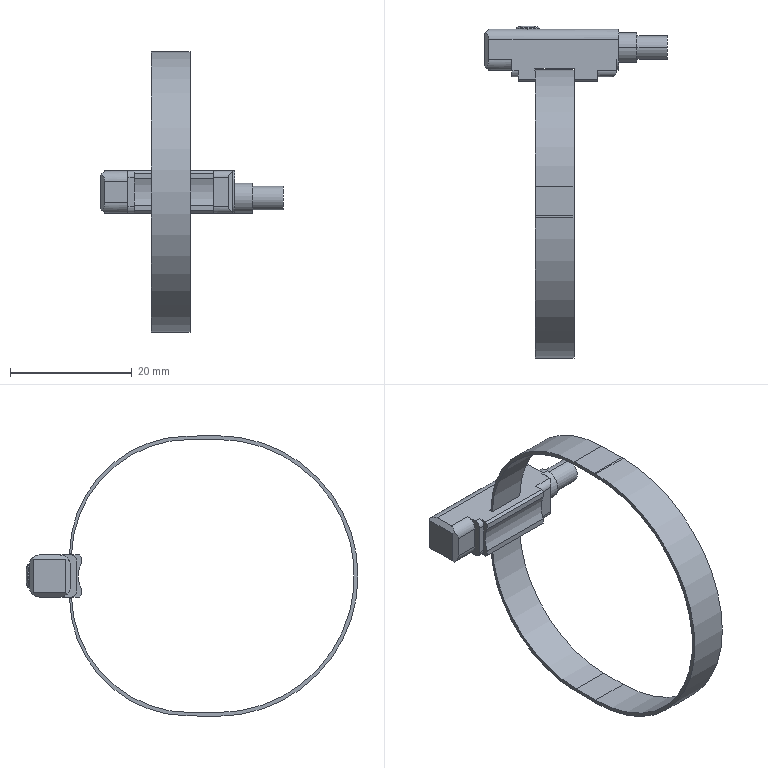Part | SolidWorks | features BaseBody 1 | 1 solid | 67 faces | box 30 x 54.5 x 46 mm | volume 1772 mm3 | plane 39 | cylinder 25 | spline 3 | commonest cylinder face diameters 3.4 x6 2 x4 39 x4 46 x3 3.8 x2 3.9 x2